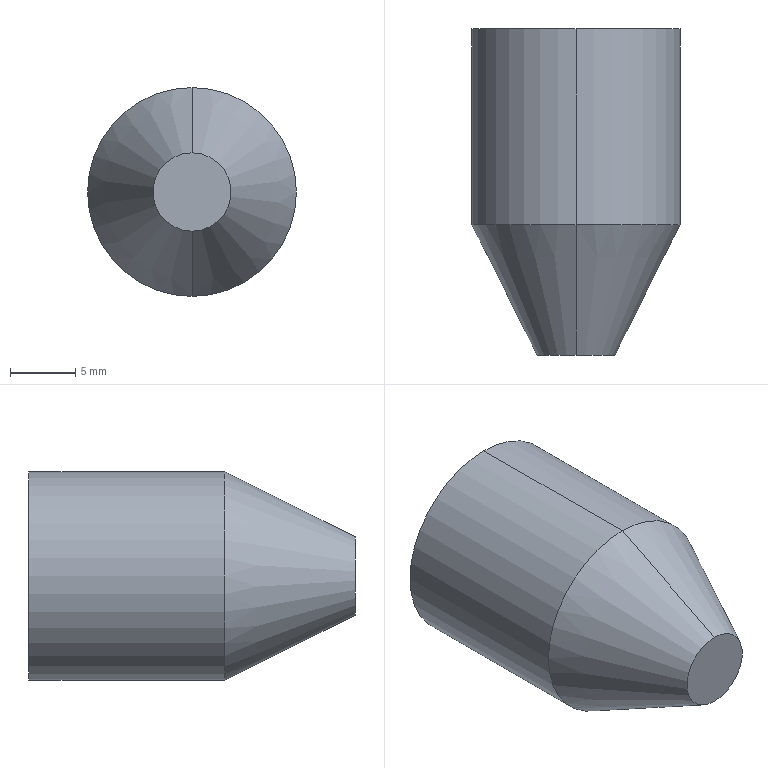Part | SolidWorks | features Chamfer 1, Extrusion 1, RevCut 1 | 1 solid | 9 faces | box 16 x 25 x 16 mm | volume 2776 mm3 | cone 4 | plane 3 | cylinder 2 | commonest cylinder face diameters 16 x2
STEP:
#1=CARTESIAN_POINT('',(0.,14.,-5.75));
#2=VERTEX_POINT('',#1);
#3=CARTESIAN_POINT('',(0.,14.,5.75));
#4=VERTEX_POINT('',#3);
#5=CARTESIAN_POINT('',(0.,14.,0.));
#6=DIRECTION('',(0.,1.,0.));
#7=DIRECTION('',(0.,0.,1.));
#8=AXIS2_PLACEMENT_3D('',#5,#6,#7);
#9=CIRCLE('',#8,5.75);
#10=EDGE_CURVE('',#2,#4,#9,.T.);
#11=ORIENTED_EDGE('',*,*,#10,.F.);
#12=CARTESIAN_POINT('',(0.,25.,-6.3));
#13=VERTEX_POINT('',#12);
#14=CARTESIAN_POINT('',(0.,14.,-5.75));
#15=DIRECTION('',(0.,0.9988,-0.04994));
#16=VECTOR('',#15,1000.);
#17=LINE('',#14,#16);
#18=EDGE_CURVE('',#2,#13,#17,.T.);
#19=ORIENTED_EDGE('',*,*,#18,.T.);
#20=CARTESIAN_POINT('',(0.,25.,6.3));
#21=VERTEX_POINT('',#20);
#22=CARTESIAN_POINT('',(0.,25.,0.));
#23=DIRECTION('',(0.,1.,0.));
#24=DIRECTION('',(0.,0.,1.));
#25=AXIS2_PLACEMENT_3D('',#22,#23,#24);
#26=CIRCLE('',#25,6.3);
#27=EDGE_CURVE('',#13,#21,#26,.T.);
#28=ORIENTED_EDGE('',*,*,#27,.T.);
#29=CARTESIAN_POINT('',(0.,14.,5.75));
#30=DIRECTION('',(0.,0.9988,0.04994));
#31=VECTOR('',#30,1000.);
#32=LINE('',#29,#31);
#33=EDGE_CURVE('',#4,#21,#32,.T.);
#34=ORIENTED_EDGE('',*,*,#33,.F.);
#35=EDGE_LOOP('',(#11,#19,#28,#34));
#36=FACE_OUTER_BOUND('',#35,.T.);
#37=CARTESIAN_POINT('',(0.,14.,0.));
#38=DIRECTION('',(0.,1.,0.));
#39=DIRECTION('',(0.,0.,1.));
#40=AXIS2_PLACEMENT_3D('',#37,#38,#39);
#41=CONICAL_SURFACE('',#40,5.75,0.04996);
#42=ADVANCED_FACE('',(#36),#41,.F.);
#43=CARTESIAN_POINT('',(0.,0.,-3.));
#44=VERTEX_POINT('',#43);
#45=CARTESIAN_POINT('',(0.,0.,3.));
#46=VERTEX_POINT('',#45);
#47=CARTESIAN_POINT('',(0.,0.,0.));
#48=DIRECTION('',(0.,-1.,0.));
#49=DIRECTION('',(0.,0.,1.));
#50=AXIS2_PLACEMENT_3D('',#47,#48,#49);
#51=CIRCLE('',#50,3.);
#52=EDGE_CURVE('',#44,#46,#51,.T.);
#53=ORIENTED_EDGE('',*,*,#52,.F.);
#54=CARTESIAN_POINT('',(0.,10.,-8.));
#55=VERTEX_POINT('',#54);
#56=CARTESIAN_POINT('',(0.,10.,-8.));
#57=DIRECTION('',(0.,0.8944,-0.4472));
#58=VECTOR('',#57,1000.);
#59=LINE('',#56,#58);
#60=EDGE_CURVE('',#44,#55,#59,.T.);
#61=ORIENTED_EDGE('',*,*,#60,.T.);
#62=CARTESIAN_POINT('',(0.,10.,8.));
#63=VERTEX_POINT('',#62);
#64=CARTESIAN_POINT('',(0.,10.,0.));
#65=DIRECTION('',(0.,1.,0.));
#66=DIRECTION('',(0.,0.,1.));
#67=AXIS2_PLACEMENT_3D('',#64,#65,#66);
#68=CIRCLE('',#67,8.);
#69=EDGE_CURVE('',#63,#55,#68,.T.);
#70=ORIENTED_EDGE('',*,*,#69,.F.);
#71=CARTESIAN_POINT('',(0.,10.,8.));
#72=DIRECTION('',(0.,0.8944,0.4472));
#73=VECTOR('',#72,1000.);
#74=LINE('',#71,#73);
#75=EDGE_CURVE('',#46,#63,#74,.T.);
#76=ORIENTED_EDGE('',*,*,#75,.F.);
#77=EDGE_LOOP('',(#53,#61,#70,#76));
#78=FACE_OUTER_BOUND('',#77,.T.);
#79=CARTESIAN_POINT('',(0.,10.,0.));
#80=DIRECTION('',(0.,1.,0.));
#81=DIRECTION('',(0.,0.,1.));
#82=AXIS2_PLACEMENT_3D('',#79,#80,#81);
#83=CONICAL_SURFACE('',#82,8.,0.4636);
#84=ADVANCED_FACE('',(#78),#83,.T.);
#85=CARTESIAN_POINT('',(0.,25.,8.));
#86=VERTEX_POINT('',#85);
#87=CARTESIAN_POINT('',(0.,25.,-8.));
#88=VERTEX_POINT('',#87);
#89=CARTESIAN_POINT('',(0.,25.,0.));
#90=DIRECTION('',(0.,1.,0.));
#91=DIRECTION('',(0.,0.,1.));
#92=AXIS2_PLACEMENT_3D('',#89,#90,#91);
#93=CIRCLE('',#92,8.);
#94=EDGE_CURVE('',#86,#88,#93,.T.);
#95=ORIENTED_EDGE('',*,*,#94,.F.);
#96=CARTESIAN_POINT('',(0.,25.,8.));
#97=DIRECTION('',(0.,-1.,0.));
#98=VECTOR('',#97,1000.);
#99=LINE('',#96,#98);
#100=EDGE_CURVE('',#86,#63,#99,.T.);
#101=ORIENTED_EDGE('',*,*,#100,.T.);
#102=ORIENTED_EDGE('',*,*,#69,.T.);
#103=CARTESIAN_POINT('',(0.,25.,-8.));
#104=DIRECTION('',(0.,-1.,0.));
#105=VECTOR('',#104,1000.);
#106=LINE('',#103,#105);
#107=EDGE_CURVE('',#88,#55,#106,.T.);
#108=ORIENTED_EDGE('',*,*,#107,.F.);
#109=EDGE_LOOP('',(#95,#101,#102,#108));
#110=FACE_OUTER_BOUND('',#109,.T.);
#111=CARTESIAN_POINT('',(0.,25.,0.));
#112=DIRECTION('',(0.,-1.,0.));
#113=DIRECTION('',(0.,0.,-1.));
#114=AXIS2_PLACEMENT_3D('',#111,#112,#113);
#115=CYLINDRICAL_SURFACE('',#114,8.);
#116=ADVANCED_FACE('',(#110),#115,.T.);
#117=ORIENTED_EDGE('',*,*,#100,.F.);
#118=CARTESIAN_POINT('',(0.,25.,0.));
#119=DIRECTION('',(0.,1.,0.));
#120=DIRECTION('',(0.,0.,1.));
#121=AXIS2_PLACEMENT_3D('',#118,#119,#120);
#122=CIRCLE('',#121,8.);
#123=EDGE_CURVE('',#88,#86,#122,.T.);
#124=ORIENTED_EDGE('',*,*,#123,.F.);
#125=ORIENTED_EDGE('',*,*,#107,.T.);
#126=CARTESIAN_POINT('',(0.,10.,0.));
#127=DIRECTION('',(0.,1.,0.));
#128=DIRECTION('',(0.,0.,1.));
#129=AXIS2_PLACEMENT_3D('',#126,#127,#128);
#130=CIRCLE('',#129,8.);
#131=EDGE_CURVE('',#55,#63,#130,.T.);
#132=ORIENTED_EDGE('',*,*,#131,.T.);
#133=EDGE_LOOP('',(#117,#124,#125,#132));
#134=FACE_OUTER_BOUND('',#133,.T.);
#135=CARTESIAN_POINT('',(0.,25.,0.));
#136=DIRECTION('',(0.,-1.,0.));
#137=DIRECTION('',(0.,0.,-1.));
#138=AXIS2_PLACEMENT_3D('',#135,#136,#137);
#139=CYLINDRICAL_SURFACE('',#138,8.);
#140=ADVANCED_FACE('',(#134),#139,.T.);
#141=CARTESIAN_POINT('',(0.,25.,0.));
#142=DIRECTION('',(0.,1.,0.));
#143=DIRECTION('',(0.,0.,1.));
#144=AXIS2_PLACEMENT_3D('',#141,#142,#143);
#145=CIRCLE('',#144,6.3);
#146=EDGE_CURVE('',#21,#13,#145,.T.);
#147=ORIENTED_EDGE('',*,*,#146,.F.);
#148=ORIENTED_EDGE('',*,*,#27,.F.);
#149=EDGE_LOOP('',(#147,#148));
#150=FACE_BOUND('',#149,.T.);
#151=ORIENTED_EDGE('',*,*,#123,.T.);
#152=ORIENTED_EDGE('',*,*,#94,.T.);
#153=EDGE_LOOP('',(#151,#152));
#154=FACE_OUTER_BOUND('',#153,.T.);
#155=CARTESIAN_POINT('',(0.,25.,0.));
#156=DIRECTION('',(0.,1.,0.));
#157=DIRECTION('',(0.,0.,1.));
#158=AXIS2_PLACEMENT_3D('',#155,#156,#157);
#159=PLANE('',#158);
#160=ADVANCED_FACE('',(#150,#154),#159,.T.);
#161=CARTESIAN_POINT('',(0.,0.,0.));
#162=DIRECTION('',(0.,-1.,0.));
#163=DIRECTION('',(0.,0.,1.));
#164=AXIS2_PLACEMENT_3D('',#161,#162,#163);
#165=CIRCLE('',#164,3.);
#166=EDGE_CURVE('',#46,#44,#165,.T.);
#167=ORIENTED_EDGE('',*,*,#166,.T.);
#168=ORIENTED_EDGE('',*,*,#52,.T.);
#169=EDGE_LOOP('',(#167,#168));
#170=FACE_OUTER_BOUND('',#169,.T.);
#171=CARTESIAN_POINT('',(0.,0.,0.));
#172=DIRECTION('',(0.,1.,0.));
#173=DIRECTION('',(0.,0.,1.));
#174=AXIS2_PLACEMENT_3D('',#171,#172,#173);
#175=PLANE('',#174);
#176=ADVANCED_FACE('',(#170),#175,.F.);
#177=ORIENTED_EDGE('',*,*,#60,.F.);
#178=ORIENTED_EDGE('',*,*,#166,.F.);
#179=ORIENTED_EDGE('',*,*,#75,.T.);
#180=ORIENTED_EDGE('',*,*,#131,.F.);
#181=EDGE_LOOP('',(#177,#178,#179,#180));
#182=FACE_OUTER_BOUND('',#181,.T.);
#183=CARTESIAN_POINT('',(0.,10.,0.));
#184=DIRECTION('',(0.,1.,0.));
#185=DIRECTION('',(0.,0.,1.));
#186=AXIS2_PLACEMENT_3D('',#183,#184,#185);
#187=CONICAL_SURFACE('',#186,8.,0.4636);
#188=ADVANCED_FACE('',(#182),#187,.T.);
#189=ORIENTED_EDGE('',*,*,#18,.F.);
#190=CARTESIAN_POINT('',(0.,14.,0.));
#191=DIRECTION('',(0.,1.,0.));
#192=DIRECTION('',(0.,0.,1.));
#193=AXIS2_PLACEMENT_3D('',#190,#191,#192);
#194=CIRCLE('',#193,5.75);
#195=EDGE_CURVE('',#4,#2,#194,.T.);
#196=ORIENTED_EDGE('',*,*,#195,.F.);
#197=ORIENTED_EDGE('',*,*,#33,.T.);
#198=ORIENTED_EDGE('',*,*,#146,.T.);
#199=EDGE_LOOP('',(#189,#196,#197,#198));
#200=FACE_OUTER_BOUND('',#199,.T.);
#201=CARTESIAN_POINT('',(0.,14.,0.));
#202=DIRECTION('',(0.,1.,0.));
#203=DIRECTION('',(0.,0.,1.));
#204=AXIS2_PLACEMENT_3D('',#201,#202,#203);
#205=CONICAL_SURFACE('',#204,5.75,0.04996);
#206=ADVANCED_FACE('',(#200),#205,.F.);
#207=ORIENTED_EDGE('',*,*,#195,.T.);
#208=ORIENTED_EDGE('',*,*,#10,.T.);
#209=EDGE_LOOP('',(#207,#208));
#210=FACE_OUTER_BOUND('',#209,.T.);
#211=CARTESIAN_POINT('',(0.,14.,-5.75));
#212=DIRECTION('',(0.,1.,0.));
#213=DIRECTION('',(0.,0.,1.));
#214=AXIS2_PLACEMENT_3D('',#211,#212,#213);
#215=PLANE('',#214);
#216=ADVANCED_FACE('',(#210),#215,.T.);
#217=CLOSED_SHELL('',(#42,#84,#116,#140,#160,#176,#188,#206,#216));
#218=MANIFOLD_SOLID_BREP('',#217);
#219=CARTESIAN_POINT('',(0.,0.,0.));
#220=DIRECTION('',(0.,0.,1.));
#221=DIRECTION('',(1.,0.,0.));
#222=AXIS2_PLACEMENT_3D('',#219,#220,#221);
#223=(LENGTH_UNIT()NAMED_UNIT(*)SI_UNIT(.MILLI.,.METRE.));
#224=UNCERTAINTY_MEASURE_WITH_UNIT(LENGTH_MEASURE(0.00001),#223,'','');
#225=(NAMED_UNIT(*)PLANE_ANGLE_UNIT()SI_UNIT($,.RADIAN.));
#226=(NAMED_UNIT(*)SI_UNIT($,.STERADIAN.)SOLID_ANGLE_UNIT());
#227=(GEOMETRIC_REPRESENTATION_CONTEXT(3)GLOBAL_UNCERTAINTY_ASSIGNED_CONTEXT((#224))GLOBAL_UNIT_ASSIGNED_CONTEXT((#223,#225,#226))REPRESENTATION_CONTEXT('',''));
#228=ADVANCED_BREP_SHAPE_REPRESENTATION('',(#218,#222),#227);